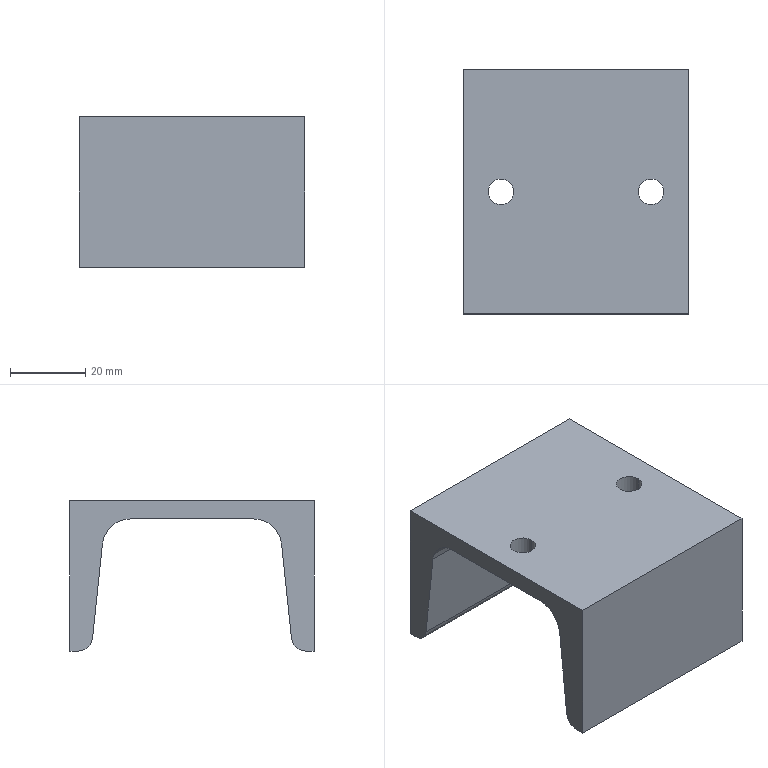Part | SolidWorks | features 3DProfileFeature 2, HoleWzd 1, WeldMemberFeat 1, WeldmentFeature 1 | 1 solid | 18 faces | box 60 x 65 x 40 mm | volume 50891 mm3 | plane 10 | cylinder 8 | commonest cylinder face diameters 6.8 x4 7.6 x2 15 x2
STEP:
#1=CARTESIAN_POINT('',(6.6,32.5,-4.8));
#2=VERTEX_POINT('',#1);
#3=CARTESIAN_POINT('',(13.4,32.5,-4.8));
#4=VERTEX_POINT('',#3);
#5=CARTESIAN_POINT('',(10.,32.5,-4.8));
#6=DIRECTION('',(0.,0.,1.));
#7=DIRECTION('',(1.,0.,0.));
#8=AXIS2_PLACEMENT_3D('',#5,#6,#7);
#9=CIRCLE('',#8,3.4);
#10=EDGE_CURVE('',#2,#4,#9,.T.);
#11=ORIENTED_EDGE('',*,*,#10,.F.);
#12=CARTESIAN_POINT('',(6.6,32.5,0.));
#13=VERTEX_POINT('',#12);
#14=CARTESIAN_POINT('',(6.6,32.5,0.));
#15=DIRECTION('',(0.,0.,1.));
#16=VECTOR('',#15,1000.);
#17=LINE('',#14,#16);
#18=EDGE_CURVE('',#2,#13,#17,.T.);
#19=ORIENTED_EDGE('',*,*,#18,.T.);
#20=CARTESIAN_POINT('',(13.4,32.5,0.));
#21=VERTEX_POINT('',#20);
#22=CARTESIAN_POINT('',(10.,32.5,0.));
#23=DIRECTION('',(0.,0.,1.));
#24=DIRECTION('',(1.,0.,0.));
#25=AXIS2_PLACEMENT_3D('',#22,#23,#24);
#26=CIRCLE('',#25,3.4);
#27=EDGE_CURVE('',#13,#21,#26,.T.);
#28=ORIENTED_EDGE('',*,*,#27,.T.);
#29=CARTESIAN_POINT('',(13.4,32.5,0.));
#30=DIRECTION('',(0.,0.,1.));
#31=VECTOR('',#30,1000.);
#32=LINE('',#29,#31);
#33=EDGE_CURVE('',#4,#21,#32,.T.);
#34=ORIENTED_EDGE('',*,*,#33,.F.);
#35=EDGE_LOOP('',(#11,#19,#28,#34));
#36=FACE_OUTER_BOUND('',#35,.T.);
#37=CARTESIAN_POINT('',(10.,32.5,0.));
#38=DIRECTION('',(0.,0.,1.));
#39=DIRECTION('',(1.,0.,0.));
#40=AXIS2_PLACEMENT_3D('',#37,#38,#39);
#41=CYLINDRICAL_SURFACE('',#40,3.4);
#42=ADVANCED_FACE('',(#36),#41,.F.);
#43=CARTESIAN_POINT('',(46.6,32.5,-4.8));
#44=VERTEX_POINT('',#43);
#45=CARTESIAN_POINT('',(53.4,32.5,-4.8));
#46=VERTEX_POINT('',#45);
#47=CARTESIAN_POINT('',(50.,32.5,-4.8));
#48=DIRECTION('',(0.,0.,1.));
#49=DIRECTION('',(1.,0.,0.));
#50=AXIS2_PLACEMENT_3D('',#47,#48,#49);
#51=CIRCLE('',#50,3.4);
#52=EDGE_CURVE('',#44,#46,#51,.T.);
#53=ORIENTED_EDGE('',*,*,#52,.F.);
#54=CARTESIAN_POINT('',(46.6,32.5,0.));
#55=VERTEX_POINT('',#54);
#56=CARTESIAN_POINT('',(46.6,32.5,0.));
#57=DIRECTION('',(0.,0.,1.));
#58=VECTOR('',#57,1000.);
#59=LINE('',#56,#58);
#60=EDGE_CURVE('',#44,#55,#59,.T.);
#61=ORIENTED_EDGE('',*,*,#60,.T.);
#62=CARTESIAN_POINT('',(53.4,32.5,0.));
#63=VERTEX_POINT('',#62);
#64=CARTESIAN_POINT('',(50.,32.5,0.));
#65=DIRECTION('',(0.,0.,1.));
#66=DIRECTION('',(1.,0.,0.));
#67=AXIS2_PLACEMENT_3D('',#64,#65,#66);
#68=CIRCLE('',#67,3.4);
#69=EDGE_CURVE('',#55,#63,#68,.T.);
#70=ORIENTED_EDGE('',*,*,#69,.T.);
#71=CARTESIAN_POINT('',(53.4,32.5,0.));
#72=DIRECTION('',(0.,0.,1.));
#73=VECTOR('',#72,1000.);
#74=LINE('',#71,#73);
#75=EDGE_CURVE('',#46,#63,#74,.T.);
#76=ORIENTED_EDGE('',*,*,#75,.F.);
#77=EDGE_LOOP('',(#53,#61,#70,#76));
#78=FACE_OUTER_BOUND('',#77,.T.);
#79=CARTESIAN_POINT('',(50.,32.5,0.));
#80=DIRECTION('',(0.,0.,1.));
#81=DIRECTION('',(1.,0.,0.));
#82=AXIS2_PLACEMENT_3D('',#79,#80,#81);
#83=CYLINDRICAL_SURFACE('',#82,3.4);
#84=ADVANCED_FACE('',(#78),#83,.F.);
#85=CARTESIAN_POINT('',(0.,58.992,-36.597));
#86=VERTEX_POINT('',#85);
#87=CARTESIAN_POINT('',(0.,62.771,-40.));
#88=VERTEX_POINT('',#87);
#89=CARTESIAN_POINT('',(0.,62.771,-36.2));
#90=DIRECTION('',(1.,0.,0.));
#91=DIRECTION('',(0.,0.,-1.));
#92=AXIS2_PLACEMENT_3D('',#89,#90,#91);
#93=CIRCLE('',#92,3.8);
#94=EDGE_CURVE('',#86,#88,#93,.T.);
#95=ORIENTED_EDGE('',*,*,#94,.T.);
#96=CARTESIAN_POINT('',(60.,62.771,-40.));
#97=VERTEX_POINT('',#96);
#98=CARTESIAN_POINT('',(60.,62.771,-40.));
#99=DIRECTION('',(-1.,0.,0.));
#100=VECTOR('',#99,1000.);
#101=LINE('',#98,#100);
#102=EDGE_CURVE('',#97,#88,#101,.T.);
#103=ORIENTED_EDGE('',*,*,#102,.F.);
#104=CARTESIAN_POINT('',(60.,58.992,-36.597));
#105=VERTEX_POINT('',#104);
#106=CARTESIAN_POINT('',(60.,62.771,-36.2));
#107=DIRECTION('',(1.,0.,0.));
#108=DIRECTION('',(0.,0.,-1.));
#109=AXIS2_PLACEMENT_3D('',#106,#107,#108);
#110=CIRCLE('',#109,3.8);
#111=EDGE_CURVE('',#105,#97,#110,.T.);
#112=ORIENTED_EDGE('',*,*,#111,.F.);
#113=CARTESIAN_POINT('',(60.,58.992,-36.597));
#114=DIRECTION('',(-1.,0.,0.));
#115=VECTOR('',#114,1000.);
#116=LINE('',#113,#115);
#117=EDGE_CURVE('',#105,#86,#116,.T.);
#118=ORIENTED_EDGE('',*,*,#117,.T.);
#119=EDGE_LOOP('',(#95,#103,#112,#118));
#120=FACE_OUTER_BOUND('',#119,.T.);
#121=CARTESIAN_POINT('',(60.,62.771,-36.2));
#122=DIRECTION('',(-1.,0.,0.));
#123=DIRECTION('',(0.,0.,1.));
#124=AXIS2_PLACEMENT_3D('',#121,#122,#123);
#125=CYLINDRICAL_SURFACE('',#124,3.8);
#126=ADVANCED_FACE('',(#120),#125,.T.);
#127=CARTESIAN_POINT('',(0.,65.,-40.));
#128=VERTEX_POINT('',#127);
#129=CARTESIAN_POINT('',(0.,65.,-40.));
#130=DIRECTION('',(0.,1.,0.));
#131=VECTOR('',#130,1000.);
#132=LINE('',#129,#131);
#133=EDGE_CURVE('',#88,#128,#132,.T.);
#134=ORIENTED_EDGE('',*,*,#133,.T.);
#135=CARTESIAN_POINT('',(60.,65.,-40.));
#136=VERTEX_POINT('',#135);
#137=CARTESIAN_POINT('',(60.,65.,-40.));
#138=DIRECTION('',(-1.,0.,0.));
#139=VECTOR('',#138,1000.);
#140=LINE('',#137,#139);
#141=EDGE_CURVE('',#136,#128,#140,.T.);
#142=ORIENTED_EDGE('',*,*,#141,.F.);
#143=CARTESIAN_POINT('',(60.,65.,-40.));
#144=DIRECTION('',(0.,1.,0.));
#145=VECTOR('',#144,1000.);
#146=LINE('',#143,#145);
#147=EDGE_CURVE('',#97,#136,#146,.T.);
#148=ORIENTED_EDGE('',*,*,#147,.F.);
#149=ORIENTED_EDGE('',*,*,#102,.T.);
#150=EDGE_LOOP('',(#134,#142,#148,#149));
#151=FACE_OUTER_BOUND('',#150,.T.);
#152=CARTESIAN_POINT('',(60.,65.,-40.));
#153=DIRECTION('',(0.,0.,1.));
#154=DIRECTION('',(1.,0.,0.));
#155=AXIS2_PLACEMENT_3D('',#152,#153,#154);
#156=PLANE('',#155);
#157=ADVANCED_FACE('',(#151),#156,.F.);
#158=CARTESIAN_POINT('',(0.,65.,0.));
#159=VERTEX_POINT('',#158);
#160=CARTESIAN_POINT('',(0.,65.,-40.));
#161=DIRECTION('',(0.,0.,1.));
#162=VECTOR('',#161,1000.);
#163=LINE('',#160,#162);
#164=EDGE_CURVE('',#128,#159,#163,.T.);
#165=ORIENTED_EDGE('',*,*,#164,.T.);
#166=CARTESIAN_POINT('',(60.,65.,0.));
#167=VERTEX_POINT('',#166);
#168=CARTESIAN_POINT('',(60.,65.,0.));
#169=DIRECTION('',(-1.,0.,0.));
#170=VECTOR('',#169,1000.);
#171=LINE('',#168,#170);
#172=EDGE_CURVE('',#167,#159,#171,.T.);
#173=ORIENTED_EDGE('',*,*,#172,.F.);
#174=CARTESIAN_POINT('',(60.,65.,-40.));
#175=DIRECTION('',(0.,0.,1.));
#176=VECTOR('',#175,1000.);
#177=LINE('',#174,#176);
#178=EDGE_CURVE('',#136,#167,#177,.T.);
#179=ORIENTED_EDGE('',*,*,#178,.F.);
#180=ORIENTED_EDGE('',*,*,#141,.T.);
#181=EDGE_LOOP('',(#165,#173,#179,#180));
#182=FACE_OUTER_BOUND('',#181,.T.);
#183=CARTESIAN_POINT('',(60.,65.,-40.));
#184=DIRECTION('',(0.,-1.,0.));
#185=DIRECTION('',(0.,0.,-1.));
#186=AXIS2_PLACEMENT_3D('',#183,#184,#185);
#187=PLANE('',#186);
#188=ADVANCED_FACE('',(#182),#187,.F.);
#189=CARTESIAN_POINT('',(10.,32.5,0.));
#190=DIRECTION('',(0.,0.,1.));
#191=DIRECTION('',(1.,0.,0.));
#192=AXIS2_PLACEMENT_3D('',#189,#190,#191);
#193=CIRCLE('',#192,3.4);
#194=EDGE_CURVE('',#21,#13,#193,.T.);
#195=ORIENTED_EDGE('',*,*,#194,.F.);
#196=ORIENTED_EDGE('',*,*,#27,.F.);
#197=EDGE_LOOP('',(#195,#196));
#198=FACE_BOUND('',#197,.T.);
#199=CARTESIAN_POINT('',(50.,32.5,0.));
#200=DIRECTION('',(0.,0.,1.));
#201=DIRECTION('',(1.,0.,0.));
#202=AXIS2_PLACEMENT_3D('',#199,#200,#201);
#203=CIRCLE('',#202,3.4);
#204=EDGE_CURVE('',#63,#55,#203,.T.);
#205=ORIENTED_EDGE('',*,*,#204,.F.);
#206=ORIENTED_EDGE('',*,*,#69,.F.);
#207=EDGE_LOOP('',(#205,#206));
#208=FACE_BOUND('',#207,.T.);
#209=CARTESIAN_POINT('',(0.,0.,0.));
#210=VERTEX_POINT('',#209);
#211=CARTESIAN_POINT('',(0.,65.,0.));
#212=DIRECTION('',(0.,-1.,0.));
#213=VECTOR('',#212,1000.);
#214=LINE('',#211,#213);
#215=EDGE_CURVE('',#159,#210,#214,.T.);
#216=ORIENTED_EDGE('',*,*,#215,.T.);
#217=CARTESIAN_POINT('',(60.,0.,0.));
#218=VERTEX_POINT('',#217);
#219=CARTESIAN_POINT('',(60.,0.,0.));
#220=DIRECTION('',(-1.,0.,0.));
#221=VECTOR('',#220,1000.);
#222=LINE('',#219,#221);
#223=EDGE_CURVE('',#218,#210,#222,.T.);
#224=ORIENTED_EDGE('',*,*,#223,.F.);
#225=CARTESIAN_POINT('',(60.,65.,0.));
#226=DIRECTION('',(0.,-1.,0.));
#227=VECTOR('',#226,1000.);
#228=LINE('',#225,#227);
#229=EDGE_CURVE('',#167,#218,#228,.T.);
#230=ORIENTED_EDGE('',*,*,#229,.F.);
#231=ORIENTED_EDGE('',*,*,#172,.T.);
#232=EDGE_LOOP('',(#216,#224,#230,#231));
#233=FACE_OUTER_BOUND('',#232,.T.);
#234=CARTESIAN_POINT('',(60.,65.,0.));
#235=DIRECTION('',(0.,0.,-1.));
#236=DIRECTION('',(-1.,0.,0.));
#237=AXIS2_PLACEMENT_3D('',#234,#235,#236);
#238=PLANE('',#237);
#239=ADVANCED_FACE('',(#198,#208,#233),#238,.F.);
#240=CARTESIAN_POINT('',(0.,0.,-40.));
#241=VERTEX_POINT('',#240);
#242=CARTESIAN_POINT('',(0.,0.,-40.));
#243=DIRECTION('',(0.,0.,-1.));
#244=VECTOR('',#243,1000.);
#245=LINE('',#242,#244);
#246=EDGE_CURVE('',#210,#241,#245,.T.);
#247=ORIENTED_EDGE('',*,*,#246,.T.);
#248=CARTESIAN_POINT('',(60.,0.,-40.));
#249=VERTEX_POINT('',#248);
#250=CARTESIAN_POINT('',(60.,0.,-40.));
#251=DIRECTION('',(-1.,0.,0.));
#252=VECTOR('',#251,1000.);
#253=LINE('',#250,#252);
#254=EDGE_CURVE('',#249,#241,#253,.T.);
#255=ORIENTED_EDGE('',*,*,#254,.F.);
#256=CARTESIAN_POINT('',(60.,0.,-40.));
#257=DIRECTION('',(0.,0.,-1.));
#258=VECTOR('',#257,1000.);
#259=LINE('',#256,#258);
#260=EDGE_CURVE('',#218,#249,#259,.T.);
#261=ORIENTED_EDGE('',*,*,#260,.F.);
#262=ORIENTED_EDGE('',*,*,#223,.T.);
#263=EDGE_LOOP('',(#247,#255,#261,#262));
#264=FACE_OUTER_BOUND('',#263,.T.);
#265=CARTESIAN_POINT('',(60.,0.,-40.));
#266=DIRECTION('',(0.,1.,0.));
#267=DIRECTION('',(0.,0.,1.));
#268=AXIS2_PLACEMENT_3D('',#265,#266,#267);
#269=PLANE('',#268);
#270=ADVANCED_FACE('',(#264),#269,.F.);
#271=CARTESIAN_POINT('',(0.,2.229,-40.));
#272=VERTEX_POINT('',#271);
#273=CARTESIAN_POINT('',(0.,0.,-40.));
#274=DIRECTION('',(0.,1.,0.));
#275=VECTOR('',#274,1000.);
#276=LINE('',#273,#275);
#277=EDGE_CURVE('',#241,#272,#276,.T.);
#278=ORIENTED_EDGE('',*,*,#277,.T.);
#279=CARTESIAN_POINT('',(60.,2.229,-40.));
#280=VERTEX_POINT('',#279);
#281=CARTESIAN_POINT('',(60.,2.229,-40.));
#282=DIRECTION('',(-1.,0.,0.));
#283=VECTOR('',#282,1000.);
#284=LINE('',#281,#283);
#285=EDGE_CURVE('',#280,#272,#284,.T.);
#286=ORIENTED_EDGE('',*,*,#285,.F.);
#287=CARTESIAN_POINT('',(60.,0.,-40.));
#288=DIRECTION('',(0.,1.,0.));
#289=VECTOR('',#288,1000.);
#290=LINE('',#287,#289);
#291=EDGE_CURVE('',#249,#280,#290,.T.);
#292=ORIENTED_EDGE('',*,*,#291,.F.);
#293=ORIENTED_EDGE('',*,*,#254,.T.);
#294=EDGE_LOOP('',(#278,#286,#292,#293));
#295=FACE_OUTER_BOUND('',#294,.T.);
#296=CARTESIAN_POINT('',(60.,0.,-40.));
#297=DIRECTION('',(0.,0.,1.));
#298=DIRECTION('',(1.,0.,0.));
#299=AXIS2_PLACEMENT_3D('',#296,#297,#298);
#300=PLANE('',#299);
#301=ADVANCED_FACE('',(#295),#300,.F.);
#302=CARTESIAN_POINT('',(0.,6.008,-36.597));
#303=VERTEX_POINT('',#302);
#304=CARTESIAN_POINT('',(0.,2.229,-36.2));
#305=DIRECTION('',(1.,0.,0.));
#306=DIRECTION('',(0.,0.,1.));
#307=AXIS2_PLACEMENT_3D('',#304,#305,#306);
#308=CIRCLE('',#307,3.8);
#309=EDGE_CURVE('',#272,#303,#308,.T.);
#310=ORIENTED_EDGE('',*,*,#309,.T.);
#311=CARTESIAN_POINT('',(60.,6.008,-36.597));
#312=VERTEX_POINT('',#311);
#313=CARTESIAN_POINT('',(60.,6.008,-36.597));
#314=DIRECTION('',(-1.,0.,0.));
#315=VECTOR('',#314,1000.);
#316=LINE('',#313,#315);
#317=EDGE_CURVE('',#312,#303,#316,.T.);
#318=ORIENTED_EDGE('',*,*,#317,.F.);
#319=CARTESIAN_POINT('',(60.,2.229,-36.2));
#320=DIRECTION('',(1.,0.,0.));
#321=DIRECTION('',(0.,0.,1.));
#322=AXIS2_PLACEMENT_3D('',#319,#320,#321);
#323=CIRCLE('',#322,3.8);
#324=EDGE_CURVE('',#280,#312,#323,.T.);
#325=ORIENTED_EDGE('',*,*,#324,.F.);
#326=ORIENTED_EDGE('',*,*,#285,.T.);
#327=EDGE_LOOP('',(#310,#318,#325,#326));
#328=FACE_OUTER_BOUND('',#327,.T.);
#329=CARTESIAN_POINT('',(60.,2.229,-36.2));
#330=DIRECTION('',(-1.,0.,0.));
#331=DIRECTION('',(0.,0.,1.));
#332=AXIS2_PLACEMENT_3D('',#329,#330,#331);
#333=CYLINDRICAL_SURFACE('',#332,3.8);
#334=ADVANCED_FACE('',(#328),#333,.T.);
#335=CARTESIAN_POINT('',(0.,8.644,-11.516));
#336=VERTEX_POINT('',#335);
#337=CARTESIAN_POINT('',(0.,8.644,-11.516));
#338=DIRECTION('',(0.,0.1045,0.9945));
#339=VECTOR('',#338,1000.);
#340=LINE('',#337,#339);
#341=EDGE_CURVE('',#303,#336,#340,.T.);
#342=ORIENTED_EDGE('',*,*,#341,.T.);
#343=CARTESIAN_POINT('',(60.,8.644,-11.516));
#344=VERTEX_POINT('',#343);
#345=CARTESIAN_POINT('',(60.,8.644,-11.516));
#346=DIRECTION('',(-1.,0.,0.));
#347=VECTOR('',#346,1000.);
#348=LINE('',#345,#347);
#349=EDGE_CURVE('',#344,#336,#348,.T.);
#350=ORIENTED_EDGE('',*,*,#349,.F.);
#351=CARTESIAN_POINT('',(60.,8.644,-11.516));
#352=DIRECTION('',(0.,0.1045,0.9945));
#353=VECTOR('',#352,1000.);
#354=LINE('',#351,#353);
#355=EDGE_CURVE('',#312,#344,#354,.T.);
#356=ORIENTED_EDGE('',*,*,#355,.F.);
#357=ORIENTED_EDGE('',*,*,#317,.T.);
#358=EDGE_LOOP('',(#342,#350,#356,#357));
#359=FACE_OUTER_BOUND('',#358,.T.);
#360=CARTESIAN_POINT('',(60.,8.644,-11.516));
#361=DIRECTION('',(0.,-0.9945,0.1045));
#362=DIRECTION('',(0.,-0.1045,-0.9945));
#363=AXIS2_PLACEMENT_3D('',#360,#361,#362);
#364=PLANE('',#363);
#365=ADVANCED_FACE('',(#359),#364,.F.);
#366=CARTESIAN_POINT('',(0.,16.103,-4.8));
#367=VERTEX_POINT('',#366);
#368=CARTESIAN_POINT('',(0.,16.103,-12.3));
#369=DIRECTION('',(-1.,0.,0.));
#370=DIRECTION('',(0.,0.,-1.));
#371=AXIS2_PLACEMENT_3D('',#368,#369,#370);
#372=CIRCLE('',#371,7.5);
#373=EDGE_CURVE('',#336,#367,#372,.T.);
#374=ORIENTED_EDGE('',*,*,#373,.T.);
#375=CARTESIAN_POINT('',(60.,16.103,-4.8));
#376=VERTEX_POINT('',#375);
#377=CARTESIAN_POINT('',(60.,16.103,-4.8));
#378=DIRECTION('',(-1.,0.,0.));
#379=VECTOR('',#378,1000.);
#380=LINE('',#377,#379);
#381=EDGE_CURVE('',#376,#367,#380,.T.);
#382=ORIENTED_EDGE('',*,*,#381,.F.);
#383=CARTESIAN_POINT('',(60.,16.103,-12.3));
#384=DIRECTION('',(-1.,0.,0.));
#385=DIRECTION('',(0.,0.,-1.));
#386=AXIS2_PLACEMENT_3D('',#383,#384,#385);
#387=CIRCLE('',#386,7.5);
#388=EDGE_CURVE('',#344,#376,#387,.T.);
#389=ORIENTED_EDGE('',*,*,#388,.F.);
#390=ORIENTED_EDGE('',*,*,#349,.T.);
#391=EDGE_LOOP('',(#374,#382,#389,#390));
#392=FACE_OUTER_BOUND('',#391,.T.);
#393=CARTESIAN_POINT('',(60.,16.103,-12.3));
#394=DIRECTION('',(-1.,0.,0.));
#395=DIRECTION('',(0.,0.,1.));
#396=AXIS2_PLACEMENT_3D('',#393,#394,#395);
#397=CYLINDRICAL_SURFACE('',#396,7.5);
#398=ADVANCED_FACE('',(#392),#397,.F.);
#399=CARTESIAN_POINT('',(10.,32.5,-4.8));
#400=DIRECTION('',(0.,0.,1.));
#401=DIRECTION('',(1.,0.,0.));
#402=AXIS2_PLACEMENT_3D('',#399,#400,#401);
#403=CIRCLE('',#402,3.4);
#404=EDGE_CURVE('',#4,#2,#403,.T.);
#405=ORIENTED_EDGE('',*,*,#404,.T.);
#406=ORIENTED_EDGE('',*,*,#10,.T.);
#407=EDGE_LOOP('',(#405,#406));
#408=FACE_BOUND('',#407,.T.);
#409=CARTESIAN_POINT('',(50.,32.5,-4.8));
#410=DIRECTION('',(0.,0.,1.));
#411=DIRECTION('',(1.,0.,0.));
#412=AXIS2_PLACEMENT_3D('',#409,#410,#411);
#413=CIRCLE('',#412,3.4);
#414=EDGE_CURVE('',#46,#44,#413,.T.);
#415=ORIENTED_EDGE('',*,*,#414,.T.);
#416=ORIENTED_EDGE('',*,*,#52,.T.);
#417=EDGE_LOOP('',(#415,#416));
#418=FACE_BOUND('',#417,.T.);
#419=CARTESIAN_POINT('',(0.,48.897,-4.8));
#420=VERTEX_POINT('',#419);
#421=CARTESIAN_POINT('',(0.,48.897,-4.8));
#422=DIRECTION('',(0.,1.,0.));
#423=VECTOR('',#422,1000.);
#424=LINE('',#421,#423);
#425=EDGE_CURVE('',#367,#420,#424,.T.);
#426=ORIENTED_EDGE('',*,*,#425,.T.);
#427=CARTESIAN_POINT('',(60.,48.897,-4.8));
#428=VERTEX_POINT('',#427);
#429=CARTESIAN_POINT('',(60.,48.897,-4.8));
#430=DIRECTION('',(-1.,0.,0.));
#431=VECTOR('',#430,1000.);
#432=LINE('',#429,#431);
#433=EDGE_CURVE('',#428,#420,#432,.T.);
#434=ORIENTED_EDGE('',*,*,#433,.F.);
#435=CARTESIAN_POINT('',(60.,48.897,-4.8));
#436=DIRECTION('',(0.,1.,0.));
#437=VECTOR('',#436,1000.);
#438=LINE('',#435,#437);
#439=EDGE_CURVE('',#376,#428,#438,.T.);
#440=ORIENTED_EDGE('',*,*,#439,.F.);
#441=ORIENTED_EDGE('',*,*,#381,.T.);
#442=EDGE_LOOP('',(#426,#434,#440,#441));
#443=FACE_OUTER_BOUND('',#442,.T.);
#444=CARTESIAN_POINT('',(60.,48.897,-4.8));
#445=DIRECTION('',(0.,0.,1.));
#446=DIRECTION('',(1.,0.,0.));
#447=AXIS2_PLACEMENT_3D('',#444,#445,#446);
#448=PLANE('',#447);
#449=ADVANCED_FACE('',(#408,#418,#443),#448,.F.);
#450=CARTESIAN_POINT('',(0.,56.356,-11.516));
#451=VERTEX_POINT('',#450);
#452=CARTESIAN_POINT('',(0.,48.897,-12.3));
#453=DIRECTION('',(-1.,0.,0.));
#454=DIRECTION('',(0.,0.,1.));
#455=AXIS2_PLACEMENT_3D('',#452,#453,#454);
#456=CIRCLE('',#455,7.5);
#457=EDGE_CURVE('',#420,#451,#456,.T.);
#458=ORIENTED_EDGE('',*,*,#457,.T.);
#459=CARTESIAN_POINT('',(60.,56.356,-11.516));
#460=VERTEX_POINT('',#459);
#461=CARTESIAN_POINT('',(60.,56.356,-11.516));
#462=DIRECTION('',(-1.,0.,0.));
#463=VECTOR('',#462,1000.);
#464=LINE('',#461,#463);
#465=EDGE_CURVE('',#460,#451,#464,.T.);
#466=ORIENTED_EDGE('',*,*,#465,.F.);
#467=CARTESIAN_POINT('',(60.,48.897,-12.3));
#468=DIRECTION('',(-1.,0.,0.));
#469=DIRECTION('',(0.,0.,1.));
#470=AXIS2_PLACEMENT_3D('',#467,#468,#469);
#471=CIRCLE('',#470,7.5);
#472=EDGE_CURVE('',#428,#460,#471,.T.);
#473=ORIENTED_EDGE('',*,*,#472,.F.);
#474=ORIENTED_EDGE('',*,*,#433,.T.);
#475=EDGE_LOOP('',(#458,#466,#473,#474));
#476=FACE_OUTER_BOUND('',#475,.T.);
#477=CARTESIAN_POINT('',(60.,48.897,-12.3));
#478=DIRECTION('',(-1.,0.,0.));
#479=DIRECTION('',(0.,0.,1.));
#480=AXIS2_PLACEMENT_3D('',#477,#478,#479);
#481=CYLINDRICAL_SURFACE('',#480,7.5);
#482=ADVANCED_FACE('',(#476),#481,.F.);
#483=CARTESIAN_POINT('',(0.,56.356,-11.516));
#484=DIRECTION('',(0.,0.1045,-0.9945));
#485=VECTOR('',#484,1000.);
#486=LINE('',#483,#485);
#487=EDGE_CURVE('',#451,#86,#486,.T.);
#488=ORIENTED_EDGE('',*,*,#487,.T.);
#489=ORIENTED_EDGE('',*,*,#117,.F.);
#490=CARTESIAN_POINT('',(60.,56.356,-11.516));
#491=DIRECTION('',(0.,0.1045,-0.9945));
#492=VECTOR('',#491,1000.);
#493=LINE('',#490,#492);
#494=EDGE_CURVE('',#460,#105,#493,.T.);
#495=ORIENTED_EDGE('',*,*,#494,.F.);
#496=ORIENTED_EDGE('',*,*,#465,.T.);
#497=EDGE_LOOP('',(#488,#489,#495,#496));
#498=FACE_OUTER_BOUND('',#497,.T.);
#499=CARTESIAN_POINT('',(60.,56.356,-11.516));
#500=DIRECTION('',(0.,0.9945,0.1045));
#501=DIRECTION('',(0.,-0.1045,0.9945));
#502=AXIS2_PLACEMENT_3D('',#499,#500,#501);
#503=PLANE('',#502);
#504=ADVANCED_FACE('',(#498),#503,.F.);
#505=ORIENTED_EDGE('',*,*,#111,.T.);
#506=ORIENTED_EDGE('',*,*,#147,.T.);
#507=ORIENTED_EDGE('',*,*,#178,.T.);
#508=ORIENTED_EDGE('',*,*,#229,.T.);
#509=ORIENTED_EDGE('',*,*,#260,.T.);
#510=ORIENTED_EDGE('',*,*,#291,.T.);
#511=ORIENTED_EDGE('',*,*,#324,.T.);
#512=ORIENTED_EDGE('',*,*,#355,.T.);
#513=ORIENTED_EDGE('',*,*,#388,.T.);
#514=ORIENTED_EDGE('',*,*,#439,.T.);
#515=ORIENTED_EDGE('',*,*,#472,.T.);
#516=ORIENTED_EDGE('',*,*,#494,.T.);
#517=EDGE_LOOP('',(#505,#506,#507,#508,#509,#510,#511,#512,#513,#514,#515,#516));
#518=FACE_OUTER_BOUND('',#517,.T.);
#519=CARTESIAN_POINT('',(60.,62.771,-36.2));
#520=DIRECTION('',(1.,0.,0.));
#521=DIRECTION('',(0.,0.,-1.));
#522=AXIS2_PLACEMENT_3D('',#519,#520,#521);
#523=PLANE('',#522);
#524=ADVANCED_FACE('',(#518),#523,.T.);
#525=ORIENTED_EDGE('',*,*,#94,.F.);
#526=ORIENTED_EDGE('',*,*,#487,.F.);
#527=ORIENTED_EDGE('',*,*,#457,.F.);
#528=ORIENTED_EDGE('',*,*,#425,.F.);
#529=ORIENTED_EDGE('',*,*,#373,.F.);
#530=ORIENTED_EDGE('',*,*,#341,.F.);
#531=ORIENTED_EDGE('',*,*,#309,.F.);
#532=ORIENTED_EDGE('',*,*,#277,.F.);
#533=ORIENTED_EDGE('',*,*,#246,.F.);
#534=ORIENTED_EDGE('',*,*,#215,.F.);
#535=ORIENTED_EDGE('',*,*,#164,.F.);
#536=ORIENTED_EDGE('',*,*,#133,.F.);
#537=EDGE_LOOP('',(#525,#526,#527,#528,#529,#530,#531,#532,#533,#534,#535,#536));
#538=FACE_OUTER_BOUND('',#537,.T.);
#539=CARTESIAN_POINT('',(0.,62.771,-36.2));
#540=DIRECTION('',(1.,0.,0.));
#541=DIRECTION('',(0.,0.,-1.));
#542=AXIS2_PLACEMENT_3D('',#539,#540,#541);
#543=PLANE('',#542);
#544=ADVANCED_FACE('',(#538),#543,.F.);
#545=ORIENTED_EDGE('',*,*,#60,.F.);
#546=ORIENTED_EDGE('',*,*,#414,.F.);
#547=ORIENTED_EDGE('',*,*,#75,.T.);
#548=ORIENTED_EDGE('',*,*,#204,.T.);
#549=EDGE_LOOP('',(#545,#546,#547,#548));
#550=FACE_OUTER_BOUND('',#549,.T.);
#551=CARTESIAN_POINT('',(50.,32.5,0.));
#552=DIRECTION('',(0.,0.,1.));
#553=DIRECTION('',(1.,0.,0.));
#554=AXIS2_PLACEMENT_3D('',#551,#552,#553);
#555=CYLINDRICAL_SURFACE('',#554,3.4);
#556=ADVANCED_FACE('',(#550),#555,.F.);
#557=ORIENTED_EDGE('',*,*,#18,.F.);
#558=ORIENTED_EDGE('',*,*,#404,.F.);
#559=ORIENTED_EDGE('',*,*,#33,.T.);
#560=ORIENTED_EDGE('',*,*,#194,.T.);
#561=EDGE_LOOP('',(#557,#558,#559,#560));
#562=FACE_OUTER_BOUND('',#561,.T.);
#563=CARTESIAN_POINT('',(10.,32.5,0.));
#564=DIRECTION('',(0.,0.,1.));
#565=DIRECTION('',(1.,0.,0.));
#566=AXIS2_PLACEMENT_3D('',#563,#564,#565);
#567=CYLINDRICAL_SURFACE('',#566,3.4);
#568=ADVANCED_FACE('',(#562),#567,.F.);
#569=CLOSED_SHELL('',(#42,#84,#126,#157,#188,#239,#270,#301,#334,#365,#398,#449,#482,#504,#524,#544,#556,#568));
#570=MANIFOLD_SOLID_BREP('',#569);
#571=CARTESIAN_POINT('',(0.,0.,0.));
#572=DIRECTION('',(0.,0.,1.));
#573=DIRECTION('',(1.,0.,0.));
#574=AXIS2_PLACEMENT_3D('',#571,#572,#573);
#575=(LENGTH_UNIT()NAMED_UNIT(*)SI_UNIT(.MILLI.,.METRE.));
#576=UNCERTAINTY_MEASURE_WITH_UNIT(LENGTH_MEASURE(0.00001),#575,'','');
#577=(NAMED_UNIT(*)PLANE_ANGLE_UNIT()SI_UNIT($,.RADIAN.));
#578=(NAMED_UNIT(*)SI_UNIT($,.STERADIAN.)SOLID_ANGLE_UNIT());
#579=(GEOMETRIC_REPRESENTATION_CONTEXT(3)GLOBAL_UNCERTAINTY_ASSIGNED_CONTEXT((#576))GLOBAL_UNIT_ASSIGNED_CONTEXT((#575,#577,#578))REPRESENTATION_CONTEXT('',''));
#580=ADVANCED_BREP_SHAPE_REPRESENTATION('',(#570,#574),#579);